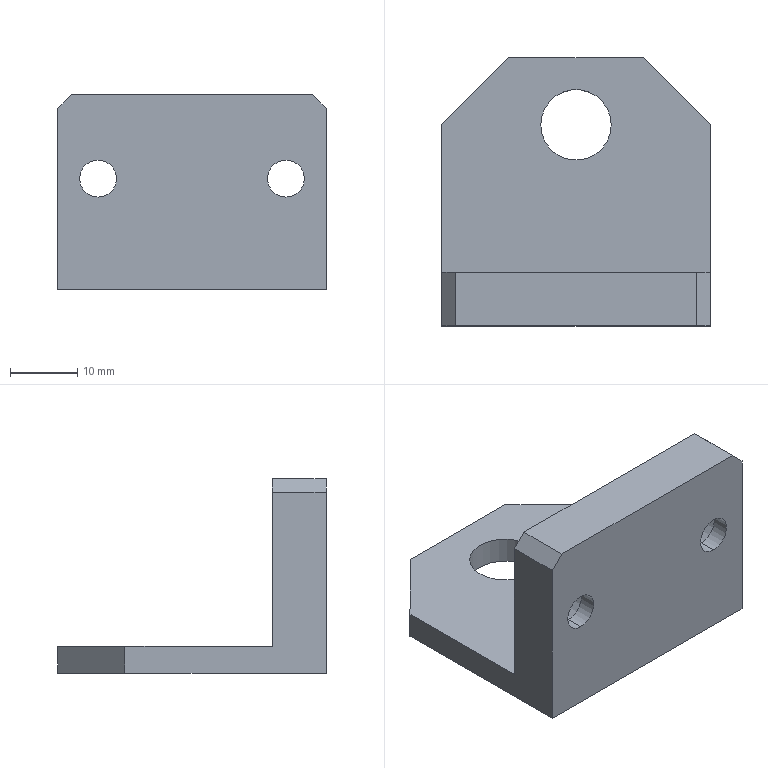Part | SolidWorks | features Chamfer 2, ICE 2, Extrusion 1, HoleWzd 1 | 1 solid | 24 faces | box 40 x 40 x 29 mm | volume 12650 mm3 | plane 14 | cylinder 10 | commonest cylinder face diameters 5.5 x4 10 x4 10.5 x2
STEP:
#1=CARTESIAN_POINT('',(-14.,-17.4,11.5));
#2=VERTEX_POINT('',#1);
#3=CARTESIAN_POINT('',(-14.,-17.4,21.5));
#4=VERTEX_POINT('',#3);
#5=CARTESIAN_POINT('',(-14.,-17.4,16.5));
#6=DIRECTION('',(0.,1.,0.));
#7=DIRECTION('',(0.,0.,1.));
#8=AXIS2_PLACEMENT_3D('',#5,#6,#7);
#9=CIRCLE('',#8,5.);
#10=EDGE_CURVE('',#2,#4,#9,.T.);
#11=ORIENTED_EDGE('',*,*,#10,.F.);
#12=CARTESIAN_POINT('',(-14.,-12.,11.5));
#13=VERTEX_POINT('',#12);
#14=CARTESIAN_POINT('',(-14.,-12.,11.5));
#15=DIRECTION('',(0.,1.,0.));
#16=VECTOR('',#15,1000.);
#17=LINE('',#14,#16);
#18=EDGE_CURVE('',#2,#13,#17,.T.);
#19=ORIENTED_EDGE('',*,*,#18,.T.);
#20=CARTESIAN_POINT('',(-14.,-12.,21.5));
#21=VERTEX_POINT('',#20);
#22=CARTESIAN_POINT('',(-14.,-12.,16.5));
#23=DIRECTION('',(0.,1.,0.));
#24=DIRECTION('',(0.,0.,1.));
#25=AXIS2_PLACEMENT_3D('',#22,#23,#24);
#26=CIRCLE('',#25,5.);
#27=EDGE_CURVE('',#13,#21,#26,.T.);
#28=ORIENTED_EDGE('',*,*,#27,.T.);
#29=CARTESIAN_POINT('',(-14.,-12.,21.5));
#30=DIRECTION('',(0.,1.,0.));
#31=VECTOR('',#30,1000.);
#32=LINE('',#29,#31);
#33=EDGE_CURVE('',#4,#21,#32,.T.);
#34=ORIENTED_EDGE('',*,*,#33,.F.);
#35=EDGE_LOOP('',(#11,#19,#28,#34));
#36=FACE_OUTER_BOUND('',#35,.T.);
#37=CARTESIAN_POINT('',(-14.,-12.,16.5));
#38=DIRECTION('',(0.,1.,0.));
#39=DIRECTION('',(0.,0.,1.));
#40=AXIS2_PLACEMENT_3D('',#37,#38,#39);
#41=CYLINDRICAL_SURFACE('',#40,5.);
#42=ADVANCED_FACE('',(#36),#41,.F.);
#43=CARTESIAN_POINT('',(-14.,-20.,13.75));
#44=VERTEX_POINT('',#43);
#45=CARTESIAN_POINT('',(-14.,-20.,19.25));
#46=VERTEX_POINT('',#45);
#47=CARTESIAN_POINT('',(-14.,-20.,16.5));
#48=DIRECTION('',(0.,1.,0.));
#49=DIRECTION('',(0.,0.,1.));
#50=AXIS2_PLACEMENT_3D('',#47,#48,#49);
#51=CIRCLE('',#50,2.75);
#52=EDGE_CURVE('',#44,#46,#51,.T.);
#53=ORIENTED_EDGE('',*,*,#52,.F.);
#54=CARTESIAN_POINT('',(-14.,-17.4,13.75));
#55=VERTEX_POINT('',#54);
#56=CARTESIAN_POINT('',(-14.,-12.,13.75));
#57=DIRECTION('',(0.,1.,0.));
#58=VECTOR('',#57,1000.);
#59=LINE('',#56,#58);
#60=EDGE_CURVE('',#44,#55,#59,.T.);
#61=ORIENTED_EDGE('',*,*,#60,.T.);
#62=CARTESIAN_POINT('',(-14.,-17.4,19.25));
#63=VERTEX_POINT('',#62);
#64=CARTESIAN_POINT('',(-14.,-17.4,16.5));
#65=DIRECTION('',(0.,1.,0.));
#66=DIRECTION('',(0.,0.,1.));
#67=AXIS2_PLACEMENT_3D('',#64,#65,#66);
#68=CIRCLE('',#67,2.75);
#69=EDGE_CURVE('',#55,#63,#68,.T.);
#70=ORIENTED_EDGE('',*,*,#69,.T.);
#71=CARTESIAN_POINT('',(-14.,-12.,19.25));
#72=DIRECTION('',(0.,1.,0.));
#73=VECTOR('',#72,1000.);
#74=LINE('',#71,#73);
#75=EDGE_CURVE('',#46,#63,#74,.T.);
#76=ORIENTED_EDGE('',*,*,#75,.F.);
#77=EDGE_LOOP('',(#53,#61,#70,#76));
#78=FACE_OUTER_BOUND('',#77,.T.);
#79=CARTESIAN_POINT('',(-14.,-12.,16.5));
#80=DIRECTION('',(0.,1.,0.));
#81=DIRECTION('',(0.,0.,1.));
#82=AXIS2_PLACEMENT_3D('',#79,#80,#81);
#83=CYLINDRICAL_SURFACE('',#82,2.75);
#84=ADVANCED_FACE('',(#78),#83,.F.);
#85=CARTESIAN_POINT('',(14.,-17.4,11.5));
#86=VERTEX_POINT('',#85);
#87=CARTESIAN_POINT('',(14.,-17.4,21.5));
#88=VERTEX_POINT('',#87);
#89=CARTESIAN_POINT('',(14.,-17.4,16.5));
#90=DIRECTION('',(0.,1.,0.));
#91=DIRECTION('',(0.,0.,1.));
#92=AXIS2_PLACEMENT_3D('',#89,#90,#91);
#93=CIRCLE('',#92,5.);
#94=EDGE_CURVE('',#86,#88,#93,.T.);
#95=ORIENTED_EDGE('',*,*,#94,.F.);
#96=CARTESIAN_POINT('',(14.,-12.,11.5));
#97=VERTEX_POINT('',#96);
#98=CARTESIAN_POINT('',(14.,-12.,11.5));
#99=DIRECTION('',(0.,1.,0.));
#100=VECTOR('',#99,1000.);
#101=LINE('',#98,#100);
#102=EDGE_CURVE('',#86,#97,#101,.T.);
#103=ORIENTED_EDGE('',*,*,#102,.T.);
#104=CARTESIAN_POINT('',(14.,-12.,21.5));
#105=VERTEX_POINT('',#104);
#106=CARTESIAN_POINT('',(14.,-12.,16.5));
#107=DIRECTION('',(0.,1.,0.));
#108=DIRECTION('',(0.,0.,1.));
#109=AXIS2_PLACEMENT_3D('',#106,#107,#108);
#110=CIRCLE('',#109,5.);
#111=EDGE_CURVE('',#97,#105,#110,.T.);
#112=ORIENTED_EDGE('',*,*,#111,.T.);
#113=CARTESIAN_POINT('',(14.,-12.,21.5));
#114=DIRECTION('',(0.,1.,0.));
#115=VECTOR('',#114,1000.);
#116=LINE('',#113,#115);
#117=EDGE_CURVE('',#88,#105,#116,.T.);
#118=ORIENTED_EDGE('',*,*,#117,.F.);
#119=EDGE_LOOP('',(#95,#103,#112,#118));
#120=FACE_OUTER_BOUND('',#119,.T.);
#121=CARTESIAN_POINT('',(14.,-12.,16.5));
#122=DIRECTION('',(0.,1.,0.));
#123=DIRECTION('',(0.,0.,1.));
#124=AXIS2_PLACEMENT_3D('',#121,#122,#123);
#125=CYLINDRICAL_SURFACE('',#124,5.);
#126=ADVANCED_FACE('',(#120),#125,.F.);
#127=CARTESIAN_POINT('',(14.,-20.,13.75));
#128=VERTEX_POINT('',#127);
#129=CARTESIAN_POINT('',(14.,-20.,19.25));
#130=VERTEX_POINT('',#129);
#131=CARTESIAN_POINT('',(14.,-20.,16.5));
#132=DIRECTION('',(0.,1.,0.));
#133=DIRECTION('',(0.,0.,1.));
#134=AXIS2_PLACEMENT_3D('',#131,#132,#133);
#135=CIRCLE('',#134,2.75);
#136=EDGE_CURVE('',#128,#130,#135,.T.);
#137=ORIENTED_EDGE('',*,*,#136,.F.);
#138=CARTESIAN_POINT('',(14.,-17.4,13.75));
#139=VERTEX_POINT('',#138);
#140=CARTESIAN_POINT('',(14.,-12.,13.75));
#141=DIRECTION('',(0.,1.,0.));
#142=VECTOR('',#141,1000.);
#143=LINE('',#140,#142);
#144=EDGE_CURVE('',#128,#139,#143,.T.);
#145=ORIENTED_EDGE('',*,*,#144,.T.);
#146=CARTESIAN_POINT('',(14.,-17.4,19.25));
#147=VERTEX_POINT('',#146);
#148=CARTESIAN_POINT('',(14.,-17.4,16.5));
#149=DIRECTION('',(0.,1.,0.));
#150=DIRECTION('',(0.,0.,1.));
#151=AXIS2_PLACEMENT_3D('',#148,#149,#150);
#152=CIRCLE('',#151,2.75);
#153=EDGE_CURVE('',#139,#147,#152,.T.);
#154=ORIENTED_EDGE('',*,*,#153,.T.);
#155=CARTESIAN_POINT('',(14.,-12.,19.25));
#156=DIRECTION('',(0.,1.,0.));
#157=VECTOR('',#156,1000.);
#158=LINE('',#155,#157);
#159=EDGE_CURVE('',#130,#147,#158,.T.);
#160=ORIENTED_EDGE('',*,*,#159,.F.);
#161=EDGE_LOOP('',(#137,#145,#154,#160));
#162=FACE_OUTER_BOUND('',#161,.T.);
#163=CARTESIAN_POINT('',(14.,-12.,16.5));
#164=DIRECTION('',(0.,1.,0.));
#165=DIRECTION('',(0.,0.,1.));
#166=AXIS2_PLACEMENT_3D('',#163,#164,#165);
#167=CYLINDRICAL_SURFACE('',#166,2.75);
#168=ADVANCED_FACE('',(#162),#167,.F.);
#169=CARTESIAN_POINT('',(-5.25,10.,0.));
#170=VERTEX_POINT('',#169);
#171=CARTESIAN_POINT('',(5.25,10.,0.));
#172=VERTEX_POINT('',#171);
#173=CARTESIAN_POINT('',(0.,10.,0.));
#174=DIRECTION('',(0.,0.,1.));
#175=DIRECTION('',(1.,0.,0.));
#176=AXIS2_PLACEMENT_3D('',#173,#174,#175);
#177=CIRCLE('',#176,5.25);
#178=EDGE_CURVE('',#170,#172,#177,.T.);
#179=ORIENTED_EDGE('',*,*,#178,.F.);
#180=CARTESIAN_POINT('',(-5.25,10.,4.));
#181=VERTEX_POINT('',#180);
#182=CARTESIAN_POINT('',(-5.25,10.,-21.));
#183=DIRECTION('',(0.,0.,1.));
#184=VECTOR('',#183,1000.);
#185=LINE('',#182,#184);
#186=EDGE_CURVE('',#170,#181,#185,.T.);
#187=ORIENTED_EDGE('',*,*,#186,.T.);
#188=CARTESIAN_POINT('',(5.25,10.,4.));
#189=VERTEX_POINT('',#188);
#190=CARTESIAN_POINT('',(0.,10.,4.));
#191=DIRECTION('',(0.,0.,1.));
#192=DIRECTION('',(1.,0.,0.));
#193=AXIS2_PLACEMENT_3D('',#190,#191,#192);
#194=CIRCLE('',#193,5.25);
#195=EDGE_CURVE('',#181,#189,#194,.T.);
#196=ORIENTED_EDGE('',*,*,#195,.T.);
#197=CARTESIAN_POINT('',(5.25,10.,-21.));
#198=DIRECTION('',(0.,0.,1.));
#199=VECTOR('',#198,1000.);
#200=LINE('',#197,#199);
#201=EDGE_CURVE('',#172,#189,#200,.T.);
#202=ORIENTED_EDGE('',*,*,#201,.F.);
#203=EDGE_LOOP('',(#179,#187,#196,#202));
#204=FACE_OUTER_BOUND('',#203,.T.);
#205=CARTESIAN_POINT('',(0.,10.,-21.));
#206=DIRECTION('',(0.,0.,1.));
#207=DIRECTION('',(1.,0.,0.));
#208=AXIS2_PLACEMENT_3D('',#205,#206,#207);
#209=CYLINDRICAL_SURFACE('',#208,5.25);
#210=ADVANCED_FACE('',(#204),#209,.F.);
#211=CARTESIAN_POINT('',(20.,-12.,27.));
#212=VERTEX_POINT('',#211);
#213=CARTESIAN_POINT('',(20.,-12.,4.));
#214=VERTEX_POINT('',#213);
#215=CARTESIAN_POINT('',(20.,-12.,29.));
#216=DIRECTION('',(0.,0.,-1.));
#217=VECTOR('',#216,1000.);
#218=LINE('',#215,#217);
#219=EDGE_CURVE('',#212,#214,#218,.T.);
#220=ORIENTED_EDGE('',*,*,#219,.F.);
#221=CARTESIAN_POINT('',(20.,-20.,27.));
#222=VERTEX_POINT('',#221);
#223=CARTESIAN_POINT('',(20.,20.,27.));
#224=DIRECTION('',(0.,-1.,0.));
#225=VECTOR('',#224,1000.);
#226=LINE('',#223,#225);
#227=EDGE_CURVE('',#212,#222,#226,.T.);
#228=ORIENTED_EDGE('',*,*,#227,.T.);
#229=CARTESIAN_POINT('',(20.,-20.,0.));
#230=VERTEX_POINT('',#229);
#231=CARTESIAN_POINT('',(20.,-20.,4.));
#232=DIRECTION('',(0.,0.,-1.));
#233=VECTOR('',#232,1000.);
#234=LINE('',#231,#233);
#235=EDGE_CURVE('',#222,#230,#234,.T.);
#236=ORIENTED_EDGE('',*,*,#235,.T.);
#237=CARTESIAN_POINT('',(20.,10.,0.));
#238=VERTEX_POINT('',#237);
#239=CARTESIAN_POINT('',(20.,20.,0.));
#240=DIRECTION('',(0.,1.,0.));
#241=VECTOR('',#240,1000.);
#242=LINE('',#239,#241);
#243=EDGE_CURVE('',#230,#238,#242,.T.);
#244=ORIENTED_EDGE('',*,*,#243,.T.);
#245=CARTESIAN_POINT('',(20.,10.,4.));
#246=VERTEX_POINT('',#245);
#247=CARTESIAN_POINT('',(20.,10.,4.));
#248=DIRECTION('',(0.,0.,1.));
#249=VECTOR('',#248,1000.);
#250=LINE('',#247,#249);
#251=EDGE_CURVE('',#238,#246,#250,.T.);
#252=ORIENTED_EDGE('',*,*,#251,.T.);
#253=CARTESIAN_POINT('',(20.,20.,4.));
#254=DIRECTION('',(0.,1.,0.));
#255=VECTOR('',#254,1000.);
#256=LINE('',#253,#255);
#257=EDGE_CURVE('',#214,#246,#256,.T.);
#258=ORIENTED_EDGE('',*,*,#257,.F.);
#259=EDGE_LOOP('',(#220,#228,#236,#244,#252,#258));
#260=FACE_OUTER_BOUND('',#259,.T.);
#261=CARTESIAN_POINT('',(20.,20.,4.));
#262=DIRECTION('',(-1.,0.,0.));
#263=DIRECTION('',(0.,-1.,0.));
#264=AXIS2_PLACEMENT_3D('',#261,#262,#263);
#265=PLANE('',#264);
#266=ADVANCED_FACE('',(#260),#265,.F.);
#267=CARTESIAN_POINT('',(10.,20.,4.));
#268=VERTEX_POINT('',#267);
#269=CARTESIAN_POINT('',(-10.,20.,4.));
#270=VERTEX_POINT('',#269);
#271=CARTESIAN_POINT('',(-20.,20.,4.));
#272=DIRECTION('',(-1.,0.,0.));
#273=VECTOR('',#272,1000.);
#274=LINE('',#271,#273);
#275=EDGE_CURVE('',#268,#270,#274,.T.);
#276=ORIENTED_EDGE('',*,*,#275,.F.);
#277=CARTESIAN_POINT('',(10.,20.,0.));
#278=VERTEX_POINT('',#277);
#279=CARTESIAN_POINT('',(10.,20.,4.));
#280=DIRECTION('',(0.,0.,-1.));
#281=VECTOR('',#280,1000.);
#282=LINE('',#279,#281);
#283=EDGE_CURVE('',#268,#278,#282,.T.);
#284=ORIENTED_EDGE('',*,*,#283,.T.);
#285=CARTESIAN_POINT('',(-10.,20.,0.));
#286=VERTEX_POINT('',#285);
#287=CARTESIAN_POINT('',(-20.,20.,0.));
#288=DIRECTION('',(-1.,0.,0.));
#289=VECTOR('',#288,1000.);
#290=LINE('',#287,#289);
#291=EDGE_CURVE('',#278,#286,#290,.T.);
#292=ORIENTED_EDGE('',*,*,#291,.T.);
#293=CARTESIAN_POINT('',(-10.,20.,4.));
#294=DIRECTION('',(0.,0.,1.));
#295=VECTOR('',#294,1000.);
#296=LINE('',#293,#295);
#297=EDGE_CURVE('',#286,#270,#296,.T.);
#298=ORIENTED_EDGE('',*,*,#297,.T.);
#299=EDGE_LOOP('',(#276,#284,#292,#298));
#300=FACE_OUTER_BOUND('',#299,.T.);
#301=CARTESIAN_POINT('',(-20.,20.,4.));
#302=DIRECTION('',(0.,-1.,0.));
#303=DIRECTION('',(0.,0.,-1.));
#304=AXIS2_PLACEMENT_3D('',#301,#302,#303);
#305=PLANE('',#304);
#306=ADVANCED_FACE('',(#300),#305,.F.);
#307=CARTESIAN_POINT('',(-20.,-20.,27.));
#308=VERTEX_POINT('',#307);
#309=CARTESIAN_POINT('',(-20.,-20.,0.));
#310=VERTEX_POINT('',#309);
#311=CARTESIAN_POINT('',(-20.,-20.,4.));
#312=DIRECTION('',(0.,0.,-1.));
#313=VECTOR('',#312,1000.);
#314=LINE('',#311,#313);
#315=EDGE_CURVE('',#308,#310,#314,.T.);
#316=ORIENTED_EDGE('',*,*,#315,.F.);
#317=CARTESIAN_POINT('',(-20.,-12.,27.));
#318=VERTEX_POINT('',#317);
#319=CARTESIAN_POINT('',(-20.,20.,27.));
#320=DIRECTION('',(0.,1.,0.));
#321=VECTOR('',#320,1000.);
#322=LINE('',#319,#321);
#323=EDGE_CURVE('',#308,#318,#322,.T.);
#324=ORIENTED_EDGE('',*,*,#323,.T.);
#325=CARTESIAN_POINT('',(-20.,-12.,4.));
#326=VERTEX_POINT('',#325);
#327=CARTESIAN_POINT('',(-20.,-12.,29.));
#328=DIRECTION('',(0.,0.,-1.));
#329=VECTOR('',#328,1000.);
#330=LINE('',#327,#329);
#331=EDGE_CURVE('',#318,#326,#330,.T.);
#332=ORIENTED_EDGE('',*,*,#331,.T.);
#333=CARTESIAN_POINT('',(-20.,10.,4.));
#334=VERTEX_POINT('',#333);
#335=CARTESIAN_POINT('',(-20.,20.,4.));
#336=DIRECTION('',(0.,-1.,0.));
#337=VECTOR('',#336,1000.);
#338=LINE('',#335,#337);
#339=EDGE_CURVE('',#334,#326,#338,.T.);
#340=ORIENTED_EDGE('',*,*,#339,.F.);
#341=CARTESIAN_POINT('',(-20.,10.,0.));
#342=VERTEX_POINT('',#341);
#343=CARTESIAN_POINT('',(-20.,10.,4.));
#344=DIRECTION('',(0.,0.,-1.));
#345=VECTOR('',#344,1000.);
#346=LINE('',#343,#345);
#347=EDGE_CURVE('',#334,#342,#346,.T.);
#348=ORIENTED_EDGE('',*,*,#347,.T.);
#349=CARTESIAN_POINT('',(-20.,20.,0.));
#350=DIRECTION('',(0.,-1.,0.));
#351=VECTOR('',#350,1000.);
#352=LINE('',#349,#351);
#353=EDGE_CURVE('',#342,#310,#352,.T.);
#354=ORIENTED_EDGE('',*,*,#353,.T.);
#355=EDGE_LOOP('',(#316,#324,#332,#340,#348,#354));
#356=FACE_OUTER_BOUND('',#355,.T.);
#357=CARTESIAN_POINT('',(-20.,20.,4.));
#358=DIRECTION('',(1.,0.,0.));
#359=DIRECTION('',(0.,1.,0.));
#360=AXIS2_PLACEMENT_3D('',#357,#358,#359);
#361=PLANE('',#360);
#362=ADVANCED_FACE('',(#356),#361,.F.);
#363=CARTESIAN_POINT('',(-14.,-20.,16.5));
#364=DIRECTION('',(0.,1.,0.));
#365=DIRECTION('',(0.,0.,1.));
#366=AXIS2_PLACEMENT_3D('',#363,#364,#365);
#367=CIRCLE('',#366,2.75);
#368=EDGE_CURVE('',#46,#44,#367,.T.);
#369=ORIENTED_EDGE('',*,*,#368,.T.);
#370=ORIENTED_EDGE('',*,*,#52,.T.);
#371=EDGE_LOOP('',(#369,#370));
#372=FACE_BOUND('',#371,.T.);
#373=CARTESIAN_POINT('',(14.,-20.,16.5));
#374=DIRECTION('',(0.,1.,0.));
#375=DIRECTION('',(0.,0.,1.));
#376=AXIS2_PLACEMENT_3D('',#373,#374,#375);
#377=CIRCLE('',#376,2.75);
#378=EDGE_CURVE('',#130,#128,#377,.T.);
#379=ORIENTED_EDGE('',*,*,#378,.T.);
#380=ORIENTED_EDGE('',*,*,#136,.T.);
#381=EDGE_LOOP('',(#379,#380));
#382=FACE_BOUND('',#381,.T.);
#383=ORIENTED_EDGE('',*,*,#235,.F.);
#384=CARTESIAN_POINT('',(18.,-20.,29.));
#385=VERTEX_POINT('',#384);
#386=CARTESIAN_POINT('',(18.,-20.,29.));
#387=DIRECTION('',(-0.7071,0.,0.7071));
#388=VECTOR('',#387,1000.);
#389=LINE('',#386,#388);
#390=EDGE_CURVE('',#222,#385,#389,.T.);
#391=ORIENTED_EDGE('',*,*,#390,.T.);
#392=CARTESIAN_POINT('',(-18.,-20.,29.));
#393=VERTEX_POINT('',#392);
#394=CARTESIAN_POINT('',(-20.,-20.,29.));
#395=DIRECTION('',(1.,0.,0.));
#396=VECTOR('',#395,1000.);
#397=LINE('',#394,#396);
#398=EDGE_CURVE('',#393,#385,#397,.T.);
#399=ORIENTED_EDGE('',*,*,#398,.F.);
#400=CARTESIAN_POINT('',(-18.,-20.,29.));
#401=DIRECTION('',(-0.7071,0.,-0.7071));
#402=VECTOR('',#401,1000.);
#403=LINE('',#400,#402);
#404=EDGE_CURVE('',#393,#308,#403,.T.);
#405=ORIENTED_EDGE('',*,*,#404,.T.);
#406=ORIENTED_EDGE('',*,*,#315,.T.);
#407=CARTESIAN_POINT('',(-20.,-20.,0.));
#408=DIRECTION('',(1.,0.,0.));
#409=VECTOR('',#408,1000.);
#410=LINE('',#407,#409);
#411=EDGE_CURVE('',#310,#230,#410,.T.);
#412=ORIENTED_EDGE('',*,*,#411,.T.);
#413=EDGE_LOOP('',(#383,#391,#399,#405,#406,#412));
#414=FACE_OUTER_BOUND('',#413,.T.);
#415=CARTESIAN_POINT('',(-20.,-20.,4.));
#416=DIRECTION('',(0.,1.,0.));
#417=DIRECTION('',(0.,0.,1.));
#418=AXIS2_PLACEMENT_3D('',#415,#416,#417);
#419=PLANE('',#418);
#420=ADVANCED_FACE('',(#372,#382,#414),#419,.F.);
#421=CARTESIAN_POINT('',(0.,10.,4.));
#422=DIRECTION('',(0.,0.,1.));
#423=DIRECTION('',(1.,0.,0.));
#424=AXIS2_PLACEMENT_3D('',#421,#422,#423);
#425=CIRCLE('',#424,5.25);
#426=EDGE_CURVE('',#189,#181,#425,.T.);
#427=ORIENTED_EDGE('',*,*,#426,.F.);
#428=ORIENTED_EDGE('',*,*,#195,.F.);
#429=EDGE_LOOP('',(#427,#428));
#430=FACE_BOUND('',#429,.T.);
#431=ORIENTED_EDGE('',*,*,#257,.T.);
#432=CARTESIAN_POINT('',(15.,15.,4.));
#433=DIRECTION('',(-0.7071,0.7071,0.));
#434=VECTOR('',#433,1000.);
#435=LINE('',#432,#434);
#436=EDGE_CURVE('',#246,#268,#435,.T.);
#437=ORIENTED_EDGE('',*,*,#436,.T.);
#438=ORIENTED_EDGE('',*,*,#275,.T.);
#439=CARTESIAN_POINT('',(-15.,15.,4.));
#440=DIRECTION('',(-0.7071,-0.7071,0.));
#441=VECTOR('',#440,1000.);
#442=LINE('',#439,#441);
#443=EDGE_CURVE('',#270,#334,#442,.T.);
#444=ORIENTED_EDGE('',*,*,#443,.T.);
#445=ORIENTED_EDGE('',*,*,#339,.T.);
#446=CARTESIAN_POINT('',(-20.,-12.,4.));
#447=DIRECTION('',(-1.,0.,0.));
#448=VECTOR('',#447,1000.);
#449=LINE('',#446,#448);
#450=EDGE_CURVE('',#214,#326,#449,.T.);
#451=ORIENTED_EDGE('',*,*,#450,.F.);
#452=EDGE_LOOP('',(#431,#437,#438,#444,#445,#451));
#453=FACE_OUTER_BOUND('',#452,.T.);
#454=CARTESIAN_POINT('',(0.,0.,4.));
#455=DIRECTION('',(0.,0.,1.));
#456=DIRECTION('',(1.,0.,0.));
#457=AXIS2_PLACEMENT_3D('',#454,#455,#456);
#458=PLANE('',#457);
#459=ADVANCED_FACE('',(#430,#453),#458,.T.);
#460=CARTESIAN_POINT('',(0.,10.,0.));
#461=DIRECTION('',(0.,0.,1.));
#462=DIRECTION('',(1.,0.,0.));
#463=AXIS2_PLACEMENT_3D('',#460,#461,#462);
#464=CIRCLE('',#463,5.25);
#465=EDGE_CURVE('',#172,#170,#464,.T.);
#466=ORIENTED_EDGE('',*,*,#465,.T.);
#467=ORIENTED_EDGE('',*,*,#178,.T.);
#468=EDGE_LOOP('',(#466,#467));
#469=FACE_BOUND('',#468,.T.);
#470=ORIENTED_EDGE('',*,*,#291,.F.);
#471=CARTESIAN_POINT('',(10.,20.,0.));
#472=DIRECTION('',(0.7071,-0.7071,0.));
#473=VECTOR('',#472,1000.);
#474=LINE('',#471,#473);
#475=EDGE_CURVE('',#278,#238,#474,.T.);
#476=ORIENTED_EDGE('',*,*,#475,.T.);
#477=ORIENTED_EDGE('',*,*,#243,.F.);
#478=ORIENTED_EDGE('',*,*,#411,.F.);
#479=ORIENTED_EDGE('',*,*,#353,.F.);
#480=CARTESIAN_POINT('',(-20.,10.,0.));
#481=DIRECTION('',(0.7071,0.7071,0.));
#482=VECTOR('',#481,1000.);
#483=LINE('',#480,#482);
#484=EDGE_CURVE('',#342,#286,#483,.T.);
#485=ORIENTED_EDGE('',*,*,#484,.T.);
#486=EDGE_LOOP('',(#470,#476,#477,#478,#479,#485));
#487=FACE_OUTER_BOUND('',#486,.T.);
#488=CARTESIAN_POINT('',(0.,0.,0.));
#489=DIRECTION('',(0.,0.,1.));
#490=DIRECTION('',(1.,0.,0.));
#491=AXIS2_PLACEMENT_3D('',#488,#489,#490);
#492=PLANE('',#491);
#493=ADVANCED_FACE('',(#469,#487),#492,.F.);
#494=CARTESIAN_POINT('',(-14.,-12.,16.5));
#495=DIRECTION('',(0.,1.,0.));
#496=DIRECTION('',(0.,0.,1.));
#497=AXIS2_PLACEMENT_3D('',#494,#495,#496);
#498=CIRCLE('',#497,5.);
#499=EDGE_CURVE('',#21,#13,#498,.T.);
#500=ORIENTED_EDGE('',*,*,#499,.F.);
#501=ORIENTED_EDGE('',*,*,#27,.F.);
#502=EDGE_LOOP('',(#500,#501));
#503=FACE_BOUND('',#502,.T.);
#504=CARTESIAN_POINT('',(14.,-12.,16.5));
#505=DIRECTION('',(0.,1.,0.));
#506=DIRECTION('',(0.,0.,1.));
#507=AXIS2_PLACEMENT_3D('',#504,#505,#506);
#508=CIRCLE('',#507,5.);
#509=EDGE_CURVE('',#105,#97,#508,.T.);
#510=ORIENTED_EDGE('',*,*,#509,.F.);
#511=ORIENTED_EDGE('',*,*,#111,.F.);
#512=EDGE_LOOP('',(#510,#511));
#513=FACE_BOUND('',#512,.T.);
#514=CARTESIAN_POINT('',(18.,-12.,29.));
#515=VERTEX_POINT('',#514);
#516=CARTESIAN_POINT('',(-18.,-12.,29.));
#517=VERTEX_POINT('',#516);
#518=CARTESIAN_POINT('',(-20.,-12.,29.));
#519=DIRECTION('',(-1.,0.,0.));
#520=VECTOR('',#519,1000.);
#521=LINE('',#518,#520);
#522=EDGE_CURVE('',#515,#517,#521,.T.);
#523=ORIENTED_EDGE('',*,*,#522,.F.);
#524=CARTESIAN_POINT('',(18.,-12.,29.));
#525=DIRECTION('',(0.7071,0.,-0.7071));
#526=VECTOR('',#525,1000.);
#527=LINE('',#524,#526);
#528=EDGE_CURVE('',#515,#212,#527,.T.);
#529=ORIENTED_EDGE('',*,*,#528,.T.);
#530=ORIENTED_EDGE('',*,*,#219,.T.);
#531=ORIENTED_EDGE('',*,*,#450,.T.);
#532=ORIENTED_EDGE('',*,*,#331,.F.);
#533=CARTESIAN_POINT('',(-18.,-12.,29.));
#534=DIRECTION('',(0.7071,0.,0.7071));
#535=VECTOR('',#534,1000.);
#536=LINE('',#533,#535);
#537=EDGE_CURVE('',#318,#517,#536,.T.);
#538=ORIENTED_EDGE('',*,*,#537,.T.);
#539=EDGE_LOOP('',(#523,#529,#530,#531,#532,#538));
#540=FACE_OUTER_BOUND('',#539,.T.);
#541=CARTESIAN_POINT('',(-20.,-12.,29.));
#542=DIRECTION('',(0.,-1.,0.));
#543=DIRECTION('',(0.,0.,-1.));
#544=AXIS2_PLACEMENT_3D('',#541,#542,#543);
#545=PLANE('',#544);
#546=ADVANCED_FACE('',(#503,#513,#540),#545,.F.);
#547=ORIENTED_EDGE('',*,*,#398,.T.);
#548=CARTESIAN_POINT('',(18.,0.,29.));
#549=DIRECTION('',(0.,1.,0.));
#550=VECTOR('',#549,1000.);
#551=LINE('',#548,#550);
#552=EDGE_CURVE('',#385,#515,#551,.T.);
#553=ORIENTED_EDGE('',*,*,#552,.T.);
#554=ORIENTED_EDGE('',*,*,#522,.T.);
#555=CARTESIAN_POINT('',(-18.,0.,29.));
#556=DIRECTION('',(0.,-1.,0.));
#557=VECTOR('',#556,1000.);
#558=LINE('',#555,#557);
#559=EDGE_CURVE('',#517,#393,#558,.T.);
#560=ORIENTED_EDGE('',*,*,#559,.T.);
#561=EDGE_LOOP('',(#547,#553,#554,#560));
#562=FACE_OUTER_BOUND('',#561,.T.);
#563=CARTESIAN_POINT('',(0.,0.,29.));
#564=DIRECTION('',(0.,0.,-1.));
#565=DIRECTION('',(-1.,0.,0.));
#566=AXIS2_PLACEMENT_3D('',#563,#564,#565);
#567=PLANE('',#566);
#568=ADVANCED_FACE('',(#562),#567,.F.);
#569=ORIENTED_EDGE('',*,*,#186,.F.);
#570=ORIENTED_EDGE('',*,*,#465,.F.);
#571=ORIENTED_EDGE('',*,*,#201,.T.);
#572=ORIENTED_EDGE('',*,*,#426,.T.);
#573=EDGE_LOOP('',(#569,#570,#571,#572));
#574=FACE_OUTER_BOUND('',#573,.T.);
#575=CARTESIAN_POINT('',(0.,10.,-21.));
#576=DIRECTION('',(0.,0.,1.));
#577=DIRECTION('',(1.,0.,0.));
#578=AXIS2_PLACEMENT_3D('',#575,#576,#577);
#579=CYLINDRICAL_SURFACE('',#578,5.25);
#580=ADVANCED_FACE('',(#574),#579,.F.);
#581=ORIENTED_EDGE('',*,*,#436,.F.);
#582=ORIENTED_EDGE('',*,*,#251,.F.);
#583=ORIENTED_EDGE('',*,*,#475,.F.);
#584=ORIENTED_EDGE('',*,*,#283,.F.);
#585=EDGE_LOOP('',(#581,#582,#583,#584));
#586=FACE_OUTER_BOUND('',#585,.T.);
#587=CARTESIAN_POINT('',(10.,20.,4.));
#588=DIRECTION('',(-0.7071,-0.7071,0.));
#589=DIRECTION('',(0.,0.,-1.));
#590=AXIS2_PLACEMENT_3D('',#587,#588,#589);
#591=PLANE('',#590);
#592=ADVANCED_FACE('',(#586),#591,.F.);
#593=ORIENTED_EDGE('',*,*,#443,.F.);
#594=ORIENTED_EDGE('',*,*,#297,.F.);
#595=ORIENTED_EDGE('',*,*,#484,.F.);
#596=ORIENTED_EDGE('',*,*,#347,.F.);
#597=EDGE_LOOP('',(#593,#594,#595,#596));
#598=FACE_OUTER_BOUND('',#597,.T.);
#599=CARTESIAN_POINT('',(-20.,10.,4.));
#600=DIRECTION('',(0.7071,-0.7071,0.));
#601=DIRECTION('',(0.,0.,-1.));
#602=AXIS2_PLACEMENT_3D('',#599,#600,#601);
#603=PLANE('',#602);
#604=ADVANCED_FACE('',(#598),#603,.F.);
#605=ORIENTED_EDGE('',*,*,#144,.F.);
#606=ORIENTED_EDGE('',*,*,#378,.F.);
#607=ORIENTED_EDGE('',*,*,#159,.T.);
#608=CARTESIAN_POINT('',(14.,-17.4,16.5));
#609=DIRECTION('',(0.,1.,0.));
#610=DIRECTION('',(0.,0.,1.));
#611=AXIS2_PLACEMENT_3D('',#608,#609,#610);
#612=CIRCLE('',#611,2.75);
#613=EDGE_CURVE('',#147,#139,#612,.T.);
#614=ORIENTED_EDGE('',*,*,#613,.T.);
#615=EDGE_LOOP('',(#605,#606,#607,#614));
#616=FACE_OUTER_BOUND('',#615,.T.);
#617=CARTESIAN_POINT('',(14.,-12.,16.5));
#618=DIRECTION('',(0.,1.,0.));
#619=DIRECTION('',(0.,0.,1.));
#620=AXIS2_PLACEMENT_3D('',#617,#618,#619);
#621=CYLINDRICAL_SURFACE('',#620,2.75);
#622=ADVANCED_FACE('',(#616),#621,.F.);
#623=ORIENTED_EDGE('',*,*,#613,.F.);
#624=ORIENTED_EDGE('',*,*,#153,.F.);
#625=EDGE_LOOP('',(#623,#624));
#626=FACE_BOUND('',#625,.T.);
#627=CARTESIAN_POINT('',(14.,-17.4,16.5));
#628=DIRECTION('',(0.,1.,0.));
#629=DIRECTION('',(0.,0.,1.));
#630=AXIS2_PLACEMENT_3D('',#627,#628,#629);
#631=CIRCLE('',#630,5.);
#632=EDGE_CURVE('',#88,#86,#631,.T.);
#633=ORIENTED_EDGE('',*,*,#632,.T.);
#634=ORIENTED_EDGE('',*,*,#94,.T.);
#635=EDGE_LOOP('',(#633,#634));
#636=FACE_OUTER_BOUND('',#635,.T.);
#637=CARTESIAN_POINT('',(16.75,-17.4,16.5));
#638=DIRECTION('',(0.,-1.,0.));
#639=DIRECTION('',(0.,0.,-1.));
#640=AXIS2_PLACEMENT_3D('',#637,#638,#639);
#641=PLANE('',#640);
#642=ADVANCED_FACE('',(#626,#636),#641,.F.);
#643=ORIENTED_EDGE('',*,*,#102,.F.);
#644=ORIENTED_EDGE('',*,*,#632,.F.);
#645=ORIENTED_EDGE('',*,*,#117,.T.);
#646=ORIENTED_EDGE('',*,*,#509,.T.);
#647=EDGE_LOOP('',(#643,#644,#645,#646));
#648=FACE_OUTER_BOUND('',#647,.T.);
#649=CARTESIAN_POINT('',(14.,-12.,16.5));
#650=DIRECTION('',(0.,1.,0.));
#651=DIRECTION('',(0.,0.,1.));
#652=AXIS2_PLACEMENT_3D('',#649,#650,#651);
#653=CYLINDRICAL_SURFACE('',#652,5.);
#654=ADVANCED_FACE('',(#648),#653,.F.);
#655=ORIENTED_EDGE('',*,*,#60,.F.);
#656=ORIENTED_EDGE('',*,*,#368,.F.);
#657=ORIENTED_EDGE('',*,*,#75,.T.);
#658=CARTESIAN_POINT('',(-14.,-17.4,16.5));
#659=DIRECTION('',(0.,1.,0.));
#660=DIRECTION('',(0.,0.,1.));
#661=AXIS2_PLACEMENT_3D('',#658,#659,#660);
#662=CIRCLE('',#661,2.75);
#663=EDGE_CURVE('',#63,#55,#662,.T.);
#664=ORIENTED_EDGE('',*,*,#663,.T.);
#665=EDGE_LOOP('',(#655,#656,#657,#664));
#666=FACE_OUTER_BOUND('',#665,.T.);
#667=CARTESIAN_POINT('',(-14.,-12.,16.5));
#668=DIRECTION('',(0.,1.,0.));
#669=DIRECTION('',(0.,0.,1.));
#670=AXIS2_PLACEMENT_3D('',#667,#668,#669);
#671=CYLINDRICAL_SURFACE('',#670,2.75);
#672=ADVANCED_FACE('',(#666),#671,.F.);
#673=ORIENTED_EDGE('',*,*,#663,.F.);
#674=ORIENTED_EDGE('',*,*,#69,.F.);
#675=EDGE_LOOP('',(#673,#674));
#676=FACE_BOUND('',#675,.T.);
#677=CARTESIAN_POINT('',(-14.,-17.4,16.5));
#678=DIRECTION('',(0.,1.,0.));
#679=DIRECTION('',(0.,0.,1.));
#680=AXIS2_PLACEMENT_3D('',#677,#678,#679);
#681=CIRCLE('',#680,5.);
#682=EDGE_CURVE('',#4,#2,#681,.T.);
#683=ORIENTED_EDGE('',*,*,#682,.T.);
#684=ORIENTED_EDGE('',*,*,#10,.T.);
#685=EDGE_LOOP('',(#683,#684));
#686=FACE_OUTER_BOUND('',#685,.T.);
#687=CARTESIAN_POINT('',(-11.25,-17.4,16.5));
#688=DIRECTION('',(0.,-1.,0.));
#689=DIRECTION('',(0.,0.,-1.));
#690=AXIS2_PLACEMENT_3D('',#687,#688,#689);
#691=PLANE('',#690);
#692=ADVANCED_FACE('',(#676,#686),#691,.F.);
#693=ORIENTED_EDGE('',*,*,#18,.F.);
#694=ORIENTED_EDGE('',*,*,#682,.F.);
#695=ORIENTED_EDGE('',*,*,#33,.T.);
#696=ORIENTED_EDGE('',*,*,#499,.T.);
#697=EDGE_LOOP('',(#693,#694,#695,#696));
#698=FACE_OUTER_BOUND('',#697,.T.);
#699=CARTESIAN_POINT('',(-14.,-12.,16.5));
#700=DIRECTION('',(0.,1.,0.));
#701=DIRECTION('',(0.,0.,1.));
#702=AXIS2_PLACEMENT_3D('',#699,#700,#701);
#703=CYLINDRICAL_SURFACE('',#702,5.);
#704=ADVANCED_FACE('',(#698),#703,.F.);
#705=ORIENTED_EDGE('',*,*,#390,.F.);
#706=ORIENTED_EDGE('',*,*,#227,.F.);
#707=ORIENTED_EDGE('',*,*,#528,.F.);
#708=ORIENTED_EDGE('',*,*,#552,.F.);
#709=EDGE_LOOP('',(#705,#706,#707,#708));
#710=FACE_OUTER_BOUND('',#709,.T.);
#711=CARTESIAN_POINT('',(18.,0.,29.));
#712=DIRECTION('',(-0.7071,0.,-0.7071));
#713=DIRECTION('',(0.,1.,0.));
#714=AXIS2_PLACEMENT_3D('',#711,#712,#713);
#715=PLANE('',#714);
#716=ADVANCED_FACE('',(#710),#715,.F.);
#717=ORIENTED_EDGE('',*,*,#537,.F.);
#718=ORIENTED_EDGE('',*,*,#323,.F.);
#719=ORIENTED_EDGE('',*,*,#404,.F.);
#720=ORIENTED_EDGE('',*,*,#559,.F.);
#721=EDGE_LOOP('',(#717,#718,#719,#720));
#722=FACE_OUTER_BOUND('',#721,.T.);
#723=CARTESIAN_POINT('',(-18.,0.,29.));
#724=DIRECTION('',(0.7071,0.,-0.7071));
#725=DIRECTION('',(0.,-1.,0.));
#726=AXIS2_PLACEMENT_3D('',#723,#724,#725);
#727=PLANE('',#726);
#728=ADVANCED_FACE('',(#722),#727,.F.);
#729=CLOSED_SHELL('',(#42,#84,#126,#168,#210,#266,#306,#362,#420,#459,#493,#546,#568,#580,#592,#604,#622,#642,#654,#672,#692,#704,#716,#728));
#730=MANIFOLD_SOLID_BREP('',#729);
#731=CARTESIAN_POINT('',(0.,0.,0.));
#732=DIRECTION('',(0.,0.,1.));
#733=DIRECTION('',(1.,0.,0.));
#734=AXIS2_PLACEMENT_3D('',#731,#732,#733);
#735=(LENGTH_UNIT()NAMED_UNIT(*)SI_UNIT(.MILLI.,.METRE.));
#736=UNCERTAINTY_MEASURE_WITH_UNIT(LENGTH_MEASURE(0.00001),#735,'','');
#737=(NAMED_UNIT(*)PLANE_ANGLE_UNIT()SI_UNIT($,.RADIAN.));
#738=(NAMED_UNIT(*)SI_UNIT($,.STERADIAN.)SOLID_ANGLE_UNIT());
#739=(GEOMETRIC_REPRESENTATION_CONTEXT(3)GLOBAL_UNCERTAINTY_ASSIGNED_CONTEXT((#736))GLOBAL_UNIT_ASSIGNED_CONTEXT((#735,#737,#738))REPRESENTATION_CONTEXT('',''));
#740=ADVANCED_BREP_SHAPE_REPRESENTATION('',(#730,#734),#739);